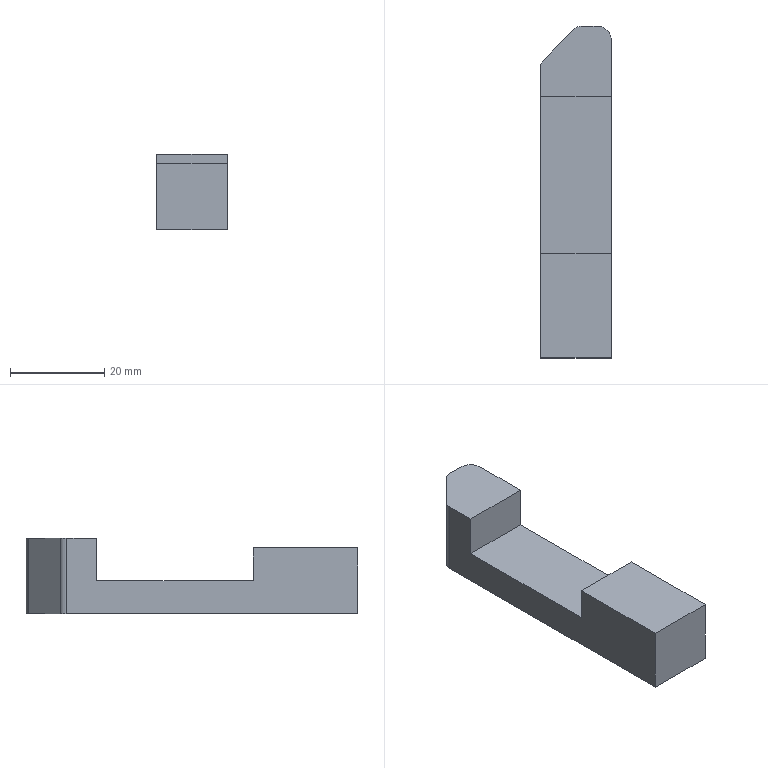Part | STEP file | 1 solid | 14 faces | box 15 x 70.5 x 16 mm | volume 11235 mm3 | plane 11 | cylinder 3 | commonest cylinder face diameters 4 x2 6 x1
STEP:
#1=CARTESIAN_POINT('',(-133.5,-144.3,5.));
#2=VERTEX_POINT('',#1);
#3=CARTESIAN_POINT('',(-133.5,-111.,5.));
#4=VERTEX_POINT('',#3);
#5=CARTESIAN_POINT('',(-133.5,-136.,5.));
#6=DIRECTION('',(0.,1.,0.));
#7=VECTOR('',#6,1.);
#8=LINE('',#5,#7);
#9=EDGE_CURVE('',#2,#4,#8,.T.);
#10=ORIENTED_EDGE('',*,*,#9,.F.);
#11=CARTESIAN_POINT('',(-118.5,-144.3,5.));
#12=VERTEX_POINT('',#11);
#13=CARTESIAN_POINT('',(-143.499,-144.3,5.));
#14=DIRECTION('',(1.,0.,0.));
#15=VECTOR('',#14,1.);
#16=LINE('',#13,#15);
#17=EDGE_CURVE('',#2,#12,#16,.T.);
#18=ORIENTED_EDGE('',*,*,#17,.T.);
#19=CARTESIAN_POINT('',(-118.5,-111.,5.));
#20=VERTEX_POINT('',#19);
#21=CARTESIAN_POINT('',(-118.5,-136.,5.));
#22=DIRECTION('',(0.,1.,0.));
#23=VECTOR('',#22,1.);
#24=LINE('',#21,#23);
#25=EDGE_CURVE('',#12,#20,#24,.T.);
#26=ORIENTED_EDGE('',*,*,#25,.T.);
#27=CARTESIAN_POINT('',(-143.499,-111.,5.));
#28=DIRECTION('',(-1.,0.,0.));
#29=VECTOR('',#28,1.);
#30=LINE('',#27,#29);
#31=EDGE_CURVE('',#20,#4,#30,.T.);
#32=ORIENTED_EDGE('',*,*,#31,.T.);
#33=EDGE_LOOP('',(#10,#18,#26,#32));
#34=FACE_OUTER_BOUND('',#33,.T.);
#35=CARTESIAN_POINT('',(-143.499,-136.,5.));
#36=DIRECTION('',(0.,0.,-1.));
#37=DIRECTION('',(-1.,0.,0.));
#38=AXIS2_PLACEMENT_3D('',#35,#36,#37);
#39=PLANE('',#38);
#40=ADVANCED_FACE('',(#34),#39,.F.);
#41=CARTESIAN_POINT('',(-118.5,-166.5,-2.));
#42=VERTEX_POINT('',#41);
#43=CARTESIAN_POINT('',(-133.5,-166.5,-2.));
#44=VERTEX_POINT('',#43);
#45=CARTESIAN_POINT('',(-145.951,-166.5,-2.));
#46=DIRECTION('',(-1.,0.,0.));
#47=VECTOR('',#46,1.);
#48=LINE('',#45,#47);
#49=EDGE_CURVE('',#42,#44,#48,.T.);
#50=ORIENTED_EDGE('',*,*,#49,.T.);
#51=CARTESIAN_POINT('',(-133.5,-104.657,-2.));
#52=VERTEX_POINT('',#51);
#53=CARTESIAN_POINT('',(-133.5,-81.,-2.));
#54=DIRECTION('',(0.,-1.,0.));
#55=VECTOR('',#54,1.);
#56=LINE('',#53,#55);
#57=EDGE_CURVE('',#52,#44,#56,.T.);
#58=ORIENTED_EDGE('',*,*,#57,.F.);
#59=CARTESIAN_POINT('',(-132.914,-103.243,-2.));
#60=VERTEX_POINT('',#59);
#61=CARTESIAN_POINT('',(-131.5,-104.657,-2.));
#62=DIRECTION('',(0.,0.,1.));
#63=DIRECTION('',(-1.,0.,0.));
#64=AXIS2_PLACEMENT_3D('',#61,#62,#63);
#65=CIRCLE('',#64,2.);
#66=EDGE_CURVE('',#60,#52,#65,.T.);
#67=ORIENTED_EDGE('',*,*,#66,.F.);
#68=CARTESIAN_POINT('',(-126.257,-96.586,-2.));
#69=VERTEX_POINT('',#68);
#70=CARTESIAN_POINT('',(-143.461,-113.79,-2.));
#71=DIRECTION('',(-0.7071,-0.7071,0.));
#72=VECTOR('',#71,1.);
#73=LINE('',#70,#72);
#74=EDGE_CURVE('',#69,#60,#73,.T.);
#75=ORIENTED_EDGE('',*,*,#74,.F.);
#76=CARTESIAN_POINT('',(-124.843,-96.,-2.));
#77=VERTEX_POINT('',#76);
#78=CARTESIAN_POINT('',(-124.843,-98.,-2.));
#79=DIRECTION('',(0.,0.,1.));
#80=DIRECTION('',(-1.,0.,0.));
#81=AXIS2_PLACEMENT_3D('',#78,#79,#80);
#82=CIRCLE('',#81,2.);
#83=EDGE_CURVE('',#77,#69,#82,.T.);
#84=ORIENTED_EDGE('',*,*,#83,.F.);
#85=CARTESIAN_POINT('',(-121.5,-96.,-2.));
#86=VERTEX_POINT('',#85);
#87=CARTESIAN_POINT('',(-122.,-96.,-2.));
#88=DIRECTION('',(-1.,0.,0.));
#89=VECTOR('',#88,1.);
#90=LINE('',#87,#89);
#91=EDGE_CURVE('',#86,#77,#90,.T.);
#92=ORIENTED_EDGE('',*,*,#91,.F.);
#93=CARTESIAN_POINT('',(-118.5,-99.,-2.));
#94=VERTEX_POINT('',#93);
#95=CARTESIAN_POINT('',(-121.5,-99.,-2.));
#96=DIRECTION('',(0.,0.,1.));
#97=DIRECTION('',(-1.,0.,0.));
#98=AXIS2_PLACEMENT_3D('',#95,#96,#97);
#99=CIRCLE('',#98,3.);
#100=EDGE_CURVE('',#94,#86,#99,.T.);
#101=ORIENTED_EDGE('',*,*,#100,.F.);
#102=CARTESIAN_POINT('',(-118.5,-111.3,-2.));
#103=DIRECTION('',(0.,1.,0.));
#104=VECTOR('',#103,1.);
#105=LINE('',#102,#104);
#106=EDGE_CURVE('',#42,#94,#105,.T.);
#107=ORIENTED_EDGE('',*,*,#106,.F.);
#108=EDGE_LOOP('',(#50,#58,#67,#75,#84,#92,#101,#107));
#109=FACE_OUTER_BOUND('',#108,.T.);
#110=CARTESIAN_POINT('',(-145.951,-111.3,-2.));
#111=DIRECTION('',(0.,0.,-1.));
#112=DIRECTION('',(-1.,0.,0.));
#113=AXIS2_PLACEMENT_3D('',#110,#111,#112);
#114=PLANE('',#113);
#115=ADVANCED_FACE('',(#109),#114,.T.);
#116=CARTESIAN_POINT('',(-118.5,-99.,14.));
#117=VERTEX_POINT('',#116);
#118=CARTESIAN_POINT('',(-121.5,-96.,14.));
#119=VERTEX_POINT('',#118);
#120=CARTESIAN_POINT('',(-121.5,-99.,14.));
#121=DIRECTION('',(0.,0.,1.));
#122=DIRECTION('',(-1.,0.,0.));
#123=AXIS2_PLACEMENT_3D('',#120,#121,#122);
#124=CIRCLE('',#123,3.);
#125=EDGE_CURVE('',#117,#119,#124,.T.);
#126=ORIENTED_EDGE('',*,*,#125,.F.);
#127=CARTESIAN_POINT('',(-118.5,-99.,-11.2));
#128=DIRECTION('',(0.,0.,-1.));
#129=VECTOR('',#128,1.);
#130=LINE('',#127,#129);
#131=EDGE_CURVE('',#117,#94,#130,.T.);
#132=ORIENTED_EDGE('',*,*,#131,.T.);
#133=ORIENTED_EDGE('',*,*,#100,.T.);
#134=CARTESIAN_POINT('',(-121.5,-96.,8.));
#135=DIRECTION('',(0.,0.,1.));
#136=VECTOR('',#135,1.);
#137=LINE('',#134,#136);
#138=EDGE_CURVE('',#86,#119,#137,.T.);
#139=ORIENTED_EDGE('',*,*,#138,.T.);
#140=EDGE_LOOP('',(#126,#132,#133,#139));
#141=FACE_OUTER_BOUND('',#140,.T.);
#142=CARTESIAN_POINT('',(-121.5,-99.,-195.));
#143=DIRECTION('',(0.,0.,-1.));
#144=DIRECTION('',(1.,0.,0.));
#145=AXIS2_PLACEMENT_3D('',#142,#143,#144);
#146=CYLINDRICAL_SURFACE('',#145,3.);
#147=ADVANCED_FACE('',(#141),#146,.T.);
#148=CARTESIAN_POINT('',(-132.914,-103.243,14.));
#149=VERTEX_POINT('',#148);
#150=CARTESIAN_POINT('',(-133.5,-104.657,14.));
#151=VERTEX_POINT('',#150);
#152=CARTESIAN_POINT('',(-131.5,-104.657,14.));
#153=DIRECTION('',(0.,0.,1.));
#154=DIRECTION('',(-1.,0.,0.));
#155=AXIS2_PLACEMENT_3D('',#152,#153,#154);
#156=CIRCLE('',#155,2.);
#157=EDGE_CURVE('',#149,#151,#156,.T.);
#158=ORIENTED_EDGE('',*,*,#157,.F.);
#159=CARTESIAN_POINT('',(-132.914,-103.243,-11.2));
#160=DIRECTION('',(0.,0.,-1.));
#161=VECTOR('',#160,1.);
#162=LINE('',#159,#161);
#163=EDGE_CURVE('',#149,#60,#162,.T.);
#164=ORIENTED_EDGE('',*,*,#163,.T.);
#165=ORIENTED_EDGE('',*,*,#66,.T.);
#166=CARTESIAN_POINT('',(-133.5,-104.657,8.));
#167=DIRECTION('',(0.,0.,1.));
#168=VECTOR('',#167,1.);
#169=LINE('',#166,#168);
#170=EDGE_CURVE('',#52,#151,#169,.T.);
#171=ORIENTED_EDGE('',*,*,#170,.T.);
#172=EDGE_LOOP('',(#158,#164,#165,#171));
#173=FACE_OUTER_BOUND('',#172,.T.);
#174=CARTESIAN_POINT('',(-131.5,-104.657,-195.));
#175=DIRECTION('',(0.,0.,1.));
#176=DIRECTION('',(-1.,0.,0.));
#177=AXIS2_PLACEMENT_3D('',#174,#175,#176);
#178=CYLINDRICAL_SURFACE('',#177,2.);
#179=ADVANCED_FACE('',(#173),#178,.T.);
#180=CARTESIAN_POINT('',(-126.257,-96.586,14.));
#181=VERTEX_POINT('',#180);
#182=CARTESIAN_POINT('',(-143.461,-113.79,14.));
#183=DIRECTION('',(0.7071,0.7071,0.));
#184=VECTOR('',#183,1.);
#185=LINE('',#182,#184);
#186=EDGE_CURVE('',#149,#181,#185,.T.);
#187=ORIENTED_EDGE('',*,*,#186,.T.);
#188=CARTESIAN_POINT('',(-126.257,-96.586,8.));
#189=DIRECTION('',(0.,0.,1.));
#190=VECTOR('',#189,1.);
#191=LINE('',#188,#190);
#192=EDGE_CURVE('',#69,#181,#191,.T.);
#193=ORIENTED_EDGE('',*,*,#192,.F.);
#194=ORIENTED_EDGE('',*,*,#74,.T.);
#195=ORIENTED_EDGE('',*,*,#163,.F.);
#196=EDGE_LOOP('',(#187,#193,#194,#195));
#197=FACE_OUTER_BOUND('',#196,.T.);
#198=CARTESIAN_POINT('',(-132.086,-102.414,-195.));
#199=DIRECTION('',(0.7071,-0.7071,0.));
#200=DIRECTION('',(0.,0.,1.));
#201=AXIS2_PLACEMENT_3D('',#198,#199,#200);
#202=PLANE('',#201);
#203=ADVANCED_FACE('',(#197),#202,.F.);
#204=CARTESIAN_POINT('',(-124.843,-96.,14.));
#205=VERTEX_POINT('',#204);
#206=CARTESIAN_POINT('',(-124.843,-98.,14.));
#207=DIRECTION('',(0.,0.,1.));
#208=DIRECTION('',(-1.,0.,0.));
#209=AXIS2_PLACEMENT_3D('',#206,#207,#208);
#210=CIRCLE('',#209,2.);
#211=EDGE_CURVE('',#205,#181,#210,.T.);
#212=ORIENTED_EDGE('',*,*,#211,.F.);
#213=CARTESIAN_POINT('',(-124.843,-96.,-11.2));
#214=DIRECTION('',(0.,0.,-1.));
#215=VECTOR('',#214,1.);
#216=LINE('',#213,#215);
#217=EDGE_CURVE('',#205,#77,#216,.T.);
#218=ORIENTED_EDGE('',*,*,#217,.T.);
#219=ORIENTED_EDGE('',*,*,#83,.T.);
#220=ORIENTED_EDGE('',*,*,#192,.T.);
#221=EDGE_LOOP('',(#212,#218,#219,#220));
#222=FACE_OUTER_BOUND('',#221,.T.);
#223=CARTESIAN_POINT('',(-124.843,-98.,-195.));
#224=DIRECTION('',(0.,0.,-1.));
#225=DIRECTION('',(1.,0.,0.));
#226=AXIS2_PLACEMENT_3D('',#223,#224,#225);
#227=CYLINDRICAL_SURFACE('',#226,2.);
#228=ADVANCED_FACE('',(#222),#227,.T.);
#229=ORIENTED_EDGE('',*,*,#217,.F.);
#230=CARTESIAN_POINT('',(-145.951,-96.,14.));
#231=DIRECTION('',(-1.,0.,0.));
#232=VECTOR('',#231,1.);
#233=LINE('',#230,#232);
#234=EDGE_CURVE('',#119,#205,#233,.T.);
#235=ORIENTED_EDGE('',*,*,#234,.F.);
#236=ORIENTED_EDGE('',*,*,#138,.F.);
#237=ORIENTED_EDGE('',*,*,#91,.T.);
#238=EDGE_LOOP('',(#229,#235,#236,#237));
#239=FACE_OUTER_BOUND('',#238,.T.);
#240=CARTESIAN_POINT('',(-122.,-96.,-195.));
#241=DIRECTION('',(0.,-1.,0.));
#242=DIRECTION('',(0.,0.,1.));
#243=AXIS2_PLACEMENT_3D('',#240,#241,#242);
#244=PLANE('',#243);
#245=ADVANCED_FACE('',(#239),#244,.F.);
#246=CARTESIAN_POINT('',(-118.5,-111.,14.));
#247=VERTEX_POINT('',#246);
#248=CARTESIAN_POINT('',(-118.5,-111.,-195.));
#249=DIRECTION('',(0.,0.,1.));
#250=VECTOR('',#249,1.);
#251=LINE('',#248,#250);
#252=EDGE_CURVE('',#20,#247,#251,.T.);
#253=ORIENTED_EDGE('',*,*,#252,.T.);
#254=CARTESIAN_POINT('',(-133.5,-111.,14.));
#255=VERTEX_POINT('',#254);
#256=CARTESIAN_POINT('',(-145.951,-111.,14.));
#257=DIRECTION('',(1.,0.,0.));
#258=VECTOR('',#257,1.);
#259=LINE('',#256,#258);
#260=EDGE_CURVE('',#255,#247,#259,.T.);
#261=ORIENTED_EDGE('',*,*,#260,.F.);
#262=CARTESIAN_POINT('',(-133.5,-111.,9.));
#263=DIRECTION('',(0.,0.,-1.));
#264=VECTOR('',#263,1.);
#265=LINE('',#262,#264);
#266=EDGE_CURVE('',#255,#4,#265,.T.);
#267=ORIENTED_EDGE('',*,*,#266,.T.);
#268=ORIENTED_EDGE('',*,*,#31,.F.);
#269=EDGE_LOOP('',(#253,#261,#267,#268));
#270=FACE_OUTER_BOUND('',#269,.T.);
#271=CARTESIAN_POINT('',(-126.,-111.,9.));
#272=DIRECTION('',(0.,1.,0.));
#273=DIRECTION('',(0.,0.,1.));
#274=AXIS2_PLACEMENT_3D('',#271,#272,#273);
#275=PLANE('',#274);
#276=ADVANCED_FACE('',(#270),#275,.F.);
#277=CARTESIAN_POINT('',(-133.5,-144.3,12.));
#278=VERTEX_POINT('',#277);
#279=CARTESIAN_POINT('',(-133.5,-144.3,-2.));
#280=DIRECTION('',(0.,0.,1.));
#281=VECTOR('',#280,1.);
#282=LINE('',#279,#281);
#283=EDGE_CURVE('',#2,#278,#282,.T.);
#284=ORIENTED_EDGE('',*,*,#283,.T.);
#285=CARTESIAN_POINT('',(-118.5,-144.3,12.));
#286=VERTEX_POINT('',#285);
#287=CARTESIAN_POINT('',(-126.,-144.3,12.));
#288=DIRECTION('',(-1.,0.,0.));
#289=VECTOR('',#288,1.);
#290=LINE('',#287,#289);
#291=EDGE_CURVE('',#286,#278,#290,.T.);
#292=ORIENTED_EDGE('',*,*,#291,.F.);
#293=CARTESIAN_POINT('',(-118.5,-144.3,-2.));
#294=DIRECTION('',(0.,0.,1.));
#295=VECTOR('',#294,1.);
#296=LINE('',#293,#295);
#297=EDGE_CURVE('',#12,#286,#296,.T.);
#298=ORIENTED_EDGE('',*,*,#297,.F.);
#299=ORIENTED_EDGE('',*,*,#17,.F.);
#300=EDGE_LOOP('',(#284,#292,#298,#299));
#301=FACE_OUTER_BOUND('',#300,.T.);
#302=CARTESIAN_POINT('',(-170.951,-144.3,-2.));
#303=DIRECTION('',(0.,-1.,0.));
#304=DIRECTION('',(0.,0.,-1.));
#305=AXIS2_PLACEMENT_3D('',#302,#303,#304);
#306=PLANE('',#305);
#307=ADVANCED_FACE('',(#301),#306,.F.);
#308=CARTESIAN_POINT('',(-133.5,-166.5,12.));
#309=VERTEX_POINT('',#308);
#310=CARTESIAN_POINT('',(-133.5,-166.5,-195.));
#311=DIRECTION('',(0.,0.,1.));
#312=VECTOR('',#311,1.);
#313=LINE('',#310,#312);
#314=EDGE_CURVE('',#44,#309,#313,.T.);
#315=ORIENTED_EDGE('',*,*,#314,.T.);
#316=CARTESIAN_POINT('',(-133.5,-81.,12.));
#317=DIRECTION('',(0.,-1.,0.));
#318=VECTOR('',#317,1.);
#319=LINE('',#316,#318);
#320=EDGE_CURVE('',#278,#309,#319,.T.);
#321=ORIENTED_EDGE('',*,*,#320,.F.);
#322=ORIENTED_EDGE('',*,*,#283,.F.);
#323=ORIENTED_EDGE('',*,*,#9,.T.);
#324=ORIENTED_EDGE('',*,*,#266,.F.);
#325=CARTESIAN_POINT('',(-133.5,-111.3,14.));
#326=DIRECTION('',(0.,-1.,0.));
#327=VECTOR('',#326,1.);
#328=LINE('',#325,#327);
#329=EDGE_CURVE('',#151,#255,#328,.T.);
#330=ORIENTED_EDGE('',*,*,#329,.F.);
#331=ORIENTED_EDGE('',*,*,#170,.F.);
#332=ORIENTED_EDGE('',*,*,#57,.T.);
#333=EDGE_LOOP('',(#315,#321,#322,#323,#324,#330,#331,#332));
#334=FACE_OUTER_BOUND('',#333,.T.);
#335=CARTESIAN_POINT('',(-133.5,-81.,-195.));
#336=DIRECTION('',(1.,0.,0.));
#337=DIRECTION('',(0.,0.,-1.));
#338=AXIS2_PLACEMENT_3D('',#335,#336,#337);
#339=PLANE('',#338);
#340=ADVANCED_FACE('',(#334),#339,.F.);
#341=CARTESIAN_POINT('',(-118.5,-166.5,12.));
#342=VERTEX_POINT('',#341);
#343=CARTESIAN_POINT('',(-118.5,-81.,12.));
#344=DIRECTION('',(0.,1.,0.));
#345=VECTOR('',#344,1.);
#346=LINE('',#343,#345);
#347=EDGE_CURVE('',#342,#286,#346,.T.);
#348=ORIENTED_EDGE('',*,*,#347,.F.);
#349=CARTESIAN_POINT('',(-118.5,-166.5,-195.));
#350=DIRECTION('',(0.,0.,1.));
#351=VECTOR('',#350,1.);
#352=LINE('',#349,#351);
#353=EDGE_CURVE('',#42,#342,#352,.T.);
#354=ORIENTED_EDGE('',*,*,#353,.F.);
#355=ORIENTED_EDGE('',*,*,#106,.T.);
#356=ORIENTED_EDGE('',*,*,#131,.F.);
#357=CARTESIAN_POINT('',(-118.5,-81.,14.));
#358=DIRECTION('',(0.,1.,0.));
#359=VECTOR('',#358,1.);
#360=LINE('',#357,#359);
#361=EDGE_CURVE('',#247,#117,#360,.T.);
#362=ORIENTED_EDGE('',*,*,#361,.F.);
#363=ORIENTED_EDGE('',*,*,#252,.F.);
#364=ORIENTED_EDGE('',*,*,#25,.F.);
#365=ORIENTED_EDGE('',*,*,#297,.T.);
#366=EDGE_LOOP('',(#348,#354,#355,#356,#362,#363,#364,#365));
#367=FACE_OUTER_BOUND('',#366,.T.);
#368=CARTESIAN_POINT('',(-118.5,-81.,-195.));
#369=DIRECTION('',(1.,0.,0.));
#370=DIRECTION('',(0.,0.,-1.));
#371=AXIS2_PLACEMENT_3D('',#368,#369,#370);
#372=PLANE('',#371);
#373=ADVANCED_FACE('',(#367),#372,.T.);
#374=ORIENTED_EDGE('',*,*,#353,.T.);
#375=CARTESIAN_POINT('',(-126.,-166.5,12.));
#376=DIRECTION('',(1.,0.,0.));
#377=VECTOR('',#376,1.);
#378=LINE('',#375,#377);
#379=EDGE_CURVE('',#309,#342,#378,.T.);
#380=ORIENTED_EDGE('',*,*,#379,.F.);
#381=ORIENTED_EDGE('',*,*,#314,.F.);
#382=ORIENTED_EDGE('',*,*,#49,.F.);
#383=EDGE_LOOP('',(#374,#380,#381,#382));
#384=FACE_OUTER_BOUND('',#383,.T.);
#385=CARTESIAN_POINT('',(-103.5,-166.5,4.));
#386=DIRECTION('',(0.,1.,0.));
#387=DIRECTION('',(0.,0.,1.));
#388=AXIS2_PLACEMENT_3D('',#385,#386,#387);
#389=PLANE('',#388);
#390=ADVANCED_FACE('',(#384),#389,.F.);
#391=ORIENTED_EDGE('',*,*,#186,.F.);
#392=ORIENTED_EDGE('',*,*,#157,.T.);
#393=ORIENTED_EDGE('',*,*,#329,.T.);
#394=ORIENTED_EDGE('',*,*,#260,.T.);
#395=ORIENTED_EDGE('',*,*,#361,.T.);
#396=ORIENTED_EDGE('',*,*,#125,.T.);
#397=ORIENTED_EDGE('',*,*,#234,.T.);
#398=ORIENTED_EDGE('',*,*,#211,.T.);
#399=EDGE_LOOP('',(#391,#392,#393,#394,#395,#396,#397,#398));
#400=FACE_OUTER_BOUND('',#399,.T.);
#401=CARTESIAN_POINT('',(-145.951,-111.3,14.));
#402=DIRECTION('',(0.,0.,-1.));
#403=DIRECTION('',(-1.,0.,0.));
#404=AXIS2_PLACEMENT_3D('',#401,#402,#403);
#405=PLANE('',#404);
#406=ADVANCED_FACE('',(#400),#405,.F.);
#407=ORIENTED_EDGE('',*,*,#347,.T.);
#408=ORIENTED_EDGE('',*,*,#291,.T.);
#409=ORIENTED_EDGE('',*,*,#320,.T.);
#410=ORIENTED_EDGE('',*,*,#379,.T.);
#411=EDGE_LOOP('',(#407,#408,#409,#410));
#412=FACE_OUTER_BOUND('',#411,.T.);
#413=CARTESIAN_POINT('',(-126.,-146.,12.));
#414=DIRECTION('',(0.,0.,-1.));
#415=DIRECTION('',(-1.,0.,0.));
#416=AXIS2_PLACEMENT_3D('',#413,#414,#415);
#417=PLANE('',#416);
#418=ADVANCED_FACE('',(#412),#417,.F.);
#419=CLOSED_SHELL('',(#40,#115,#147,#179,#203,#228,#245,#276,#307,#340,#373,#390,#406,#418));
#420=MANIFOLD_SOLID_BREP('',#419);
#421=(LENGTH_UNIT()NAMED_UNIT(*)SI_UNIT(.MILLI.,.METRE.));
#422=UNCERTAINTY_MEASURE_WITH_UNIT(LENGTH_MEASURE(0.00002),#421,'','');
#423=(NAMED_UNIT(*)PLANE_ANGLE_UNIT()SI_UNIT($,.RADIAN.));
#424=PLANE_ANGLE_MEASURE_WITH_UNIT(PLANE_ANGLE_MEASURE(0.01745),#423);
#425=DIMENSIONAL_EXPONENTS(0.,0.,0.,0.,0.,0.,0.);
#426=(CONVERSION_BASED_UNIT('DEGREE',#424)NAMED_UNIT(#425)PLANE_ANGLE_UNIT());
#427=(NAMED_UNIT(*)SI_UNIT($,.STERADIAN.)SOLID_ANGLE_UNIT());
#428=(GEOMETRIC_REPRESENTATION_CONTEXT(3)GLOBAL_UNCERTAINTY_ASSIGNED_CONTEXT((#422))GLOBAL_UNIT_ASSIGNED_CONTEXT((#421,#426,#427))REPRESENTATION_CONTEXT('',''));
#429=ADVANCED_BREP_SHAPE_REPRESENTATION('',(#420),#428);